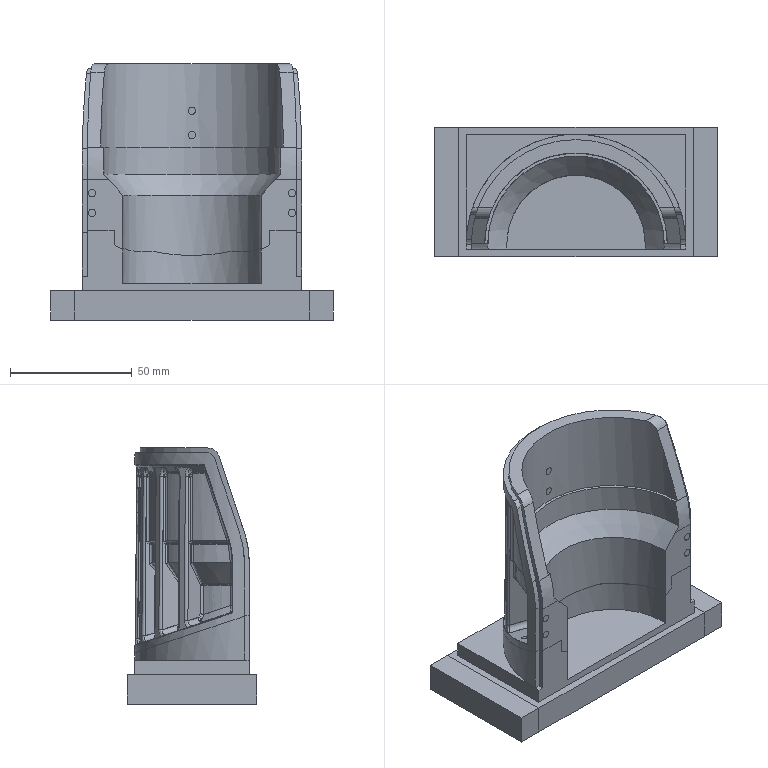NC program | NX | posted by the shop | part box 116 x 53 x 105 mm
Lines 43881 to 44922 of 572762:
T12 M6
;(T12:C-D4  D=4. R=0.)
;(XY=0.2mm Z=0.2mm)
G54 G90 D1
CYCLE832(0.04,_TOP_SURFACE_SMOOTH_ON+_ORI_SEMIFIN,1.)
CYCLE800(0,"AFMING",100000,57,0.,0.,0.,-90.,58.,0.,0.,0.,0.,-1,100.,1)
G0 X19.69 Y75.9713 S7000 M3 M8
Z103.43
X19.69 Y75.9713 Z103.43
Z35.088
G1 Z34.088 F3500.
G3 X19.4934 Y75.307 I1.003 J-.658
G1 X19.498 Y74.459
X19.485 Y73.938
G2 X19.302 Y73.304 I-2.561 J.393
X17.209 Y72.14 I-1.803 J.779
G1 X17.21 Y76.676
X19.486
X19.4934 Y75.307
X19.5154 Y74.973 Z34.094
X19.575 Y74.639 Z34.111
X19.6659 Y74.307 Z34.136
X19.784 Y73.978 Z34.166
X19.9245 Y73.653 Z34.2
X20.082 Y73.335 Z34.236
X20.434 Y72.712 Z34.3001
X20.827 Y72.073 Z34.345
X21.046 Y71.74 Z34.351
X21.2598 Y71.433 Z34.3445
X21.47 Y71.156 Z34.324
X21.676 Y70.912 Z34.292
X21.88 Y70.7056 Z34.246
X22.081 Y70.539 Z34.188
X22.208 Y70.455 Z34.145
X22.335 Y70.391 Z34.099
X22.462 Y70.349 Z34.05
X22.5896 Y70.331 Z34.002
X22.7184 Y70.339 Z33.955
X22.849 Y70.376 Z33.911
X22.981 Y70.442 Z33.871
X23.116 Y70.542 Z33.8374
X23.254 Y70.675 Z33.811
X23.395 Y70.846 Z33.795
X23.54 Y71.055 Z33.789
G3 X24.306 Y73.607 I-4.078 J2.6144
G1 Y76.676
G2 X24.675 Y77.542 I1.2 J0.0
G1 Z34.789
G0 X15.209 Y67.388
G1 Z33.789
X15.742 Y68.365
G2 X17.209 Y69.218 I1.16 J-.307
G3 X18.094 Y69.006 I5.026 J18.976
G2 X18.286 Y68.947 I-.253 J-1.173
G1 Z34.789
G0 X24.306 Y76.676 Z34.289
G1 Z33.789
X21.506
Y73.632
G2 X19.135 Y71.6517 I-2.044 J.038
X17.209 Y72.132 I3.1 J16.5422
G3 X15.705 Y71.345 I-.358 J-1.145
G1 Z34.789
G0 X15.791 Y33.438 Z34.49
G1 Z33.49
X16.008 Y33.976
G2 X17.209 Y35.175 I1.2 J-.001
G3 X18.554 Y35.201 I.037 J32.758
G1 X18.5556 Y35.216
G3 X18.627 Y38.0068 I-274.999 J8.4296
G2 X17.209 Y37.975 I-1.382 J29.926
G1 Y40.775
G3 X18.67 Y40.812 I.037 J27.1579
X18.685 Y43.353 I-275.114 J2.834
G1 X18.678 Y43.368
X18.693 Y43.374
G3 X18.903 Y43.631 I-1.417 J1.3685
G2 X17.209 Y43.575 I-1.6571 J24.3015
G1 Y46.375
G3 X19.277 Y46.471 I.037 J21.558
G1 X19.328 Y49.291
G2 X17.209 Y49.175 I-2.0824 J18.642
G1 Y51.975
G3 X19.379 Y52.118 I.037 J15.958
G1 X19.43 Y54.9575
G2 X17.209 Y54.775 I-2.184 J12.975
G1 Y57.575
G3 X19.4812 Y57.8191 I.037 J10.358
G1 X19.485 Y58.021
X19.536 Y60.069
G2 X19.534 Y60.7296 I54.9157 J.573
X17.209 Y60.375 I-2.288 J7.203
G1 Y63.175
G3 X19.589 Y63.792 I.037 J4.758
G2 X19.789 Y63.883 I.591 J-1.044
G1 Z34.49
G0 X27.205 Y77.875
G1 Z33.49
X26.777 Y77.876
G3 X25.577 Y76.676 I0.0 J-1.2
G1 Y72.434
G2 X23.121 Y70.4202 I-2.094 J.049
X19.564 Y71.126 I5.24 J35.731
G1 X19.464 Y70.86
X19.335 Y68.4635
X19.171 Y67.576
G2 X17.209 Y65.975 I-1.925 J.357
G3 X15.9867 Y64.798 I-.022 J-1.2
G1 Z34.49
G0 X28.507 Y77.819 Z34.191
G1 Z33.191
G3 X27.671 Y76.676 I.364 J-1.144
G1 Y71.791
G2 X25.513 Y69.7422 I-2.08 J.03
X23.1266 Y70.072 I.982 J15.906
G3 X22.458 Y70.025 I-.254 J-1.173
G1 Z34.191
G0 X30.015 Y77.781 Z33.892
G1 Z32.892
G3 X29.283 Y76.676 I.468 J-1.105
G1 Y71.284
G2 X27.108 Y69.227 I-2.1013 J.044
G1 X26.709 Y69.252
X26.07 Y69.3048
G2 X25.354 Y69.398 I.636 J7.696
G3 X24.708 Y69.3345 I-.21 J-1.181
G1 Z33.892
G0 X31.158 Y77.663 Z33.592
G1 Z32.592
G3 X30.64 Y76.676 I.682 J-.987
G1 Y70.845
G2 X28.714 Y68.806 I-2.042 J0.0
X26.859 Y68.917 I-.456 J7.948
G3 X26.213 Y68.855 I-.211 J-1.1813
G1 Z33.592
G0 X32.492 Y77.748 Z33.293
G1 Z32.293
G3 X31.831 Y76.676 I.54 J-1.072
G1 Y70.46
G2 X29.83 Y68.4 I-2.0607 J0.0
X28.315 Y68.456 I-.33 J11.492
G3 X27.742 Y68.375 I-.1237 J-1.194
G1 Z33.293
G0 Z36.49
X33.297 Y77.563
Z32.994
G1 Z31.994
G3 X32.905 Y76.676 I.808 J-.887
G1 Y70.107
G2 X31.073 Y68.056 I-2.064 J0.0
X30.297 Y68.033 I-.531 J4.693
X29.477 Y68.075 I-.178 J4.503
G3 X28.859 Y68.001 I-.171 J-1.188
G1 Z32.994
G0 Z36.191
X34.566 Y77.7567
Z32.695
G1 Z31.695
G3 X33.887 Y76.676 I.521 J-1.081
G1 Y69.766
G2 X32.307 Y67.794 I-2.021 J0.0
X30.503 Y67.73 I-1.072 J4.801
G3 X29.882 Y67.659 I-.178 J-1.187
G1 Z32.695
G0 Z36.191
X35.1794 Y77.554
Z32.396
G1 Z31.396
G3 X34.797 Y76.676 I.818 J-.878
G1 Y69.47
G2 X33.018 Y67.423 I-2.0666 J0.0
X32.29 Y67.368 I-.801 J5.699
G1 X32.035 Y67.363
G2 X31.522 Y67.39 I-.072 J3.478
G3 X30.92 Y67.313 I-.152 J-1.19
G1 Z32.396
G0 Z35.892
X36.232 Y77.705
Z32.097
G1 Z31.097
G3 X35.648 Y76.676 I.6165 J-1.03
G1 Y69.173
G2 X34.096 Y67.184 I-2.051 J0.0
X32.339 Y67.1 I-1.087 J4.335
G3 X31.724 Y67.032 I-.18 J-1.186
G1 Z32.097
G0 Z35.592
X36.874 Y77.592
Z31.798
G1 Z30.798
G3 X36.449 Y76.676 I.7746 J-.917
G1 Y68.902
G2 X34.283 Y66.803 I-2.134 J.034
X33.2339 Y66.7966 I-.545 J3.639
G3 X32.629 Y66.724 I-.164 J-1.189
G1 Z31.798
G0 Z35.293
X37.518 Y77.483
Z31.499
G1 Z30.499
G3 X37.2066 Y76.676 I.888 J-.807
G1 Y68.637
G2 X35.081 Y66.531 I-2.173 J.0671
X34.038 Y66.516 I-.57 J3.463
G3 X33.435 Y66.443 I-.162 J-1.189
G1 Z31.499
G0 Z34.994
X38.442 Y77.6613
Z31.2
G1 Z30.2
G3 X37.927 Y76.676 I.685 J-.985
G1 Y74.666
X37.944 Y74.2372 Z30.212
X37.9907 Y73.811 Z30.244
X38.06 Y73.389 Z30.291
X38.287 Y72.393 Z30.435
X38.525 Y71.408 Z30.562
X38.6 Y71.021 Z30.589
X38.652 Y70.649 Z30.597
X38.675 Y70.285 Z30.589
X38.666 Y69.924 Z30.562
X38.621 Y69.559 Z30.518
X38.5507 Y69.24 Z30.467
X38.451 Y68.913 Z30.408
X38.324 Y68.5805 Z30.348
X38.169 Y68.242 Z30.291
X37.988 Y67.899 Z30.244
X37.781 Y67.5517 Z30.212
X37.55 Y67.201 Z30.2
G2 X35.878 Y66.284 I-1.751 J1.209
X34.363 Y66.336 I-.644 J3.302
G1 X34.204 Y66.381
G3 X33.5108 Y66.369 I-.326 J-1.155
G1 Z31.2
G0 Z34.994
X39.108 Y77.646
Z30.901
G1 Z29.901
G3 X38.6141 Y76.676 I.706 J-.971
G1 Y68.1365
G2 X36.675 Y66.043 I-2.1266 J.025
X35.088 Y66.078 I-.72 J3.289
G1 X33.789 Y66.445
X33.5802 Y66.494 Z29.904
X33.4 Y66.5153 Z29.913
X33.246 Y66.512 Z29.926
X33.1174 Y66.485 Z29.944
X33.013 Y66.439 Z29.965
X32.931 Y66.374 Z29.987
X32.8702 Y66.294 Z30.011
X32.829 Y66.201 Z30.035
X32.806 Y66.097 Z30.058
X32.8 Y65.985 Z30.08
X32.81 Y65.866 Z30.0992
X32.8335 Y65.743 Z30.115
X32.903 Y65.53 Z30.132
X33.008 Y65.316 Z30.137
X33.146 Y65.104 Z30.129
X33.314 Y64.898 Z30.109
X33.512 Y64.701 Z30.077
X33.735 Y64.516 Z30.033
X33.984 Y64.348 Z29.978
X34.254 Y64.1981 Z29.912
X34.546 Y64.068 Z29.841
X34.86 Y63.958 Z29.77
X35.193 Y63.869 Z29.705
X35.545 Y63.801 Z29.651
X35.916 Y63.7547 Z29.615
X36.305 Y63.73 Z29.601
G3 X38.158 Y63.927 I.22 J6.75
X39.656 Y64.647 I-.9925 J3.985
G2 X39.884 Y64.784 I.728 J-.954
G1 Z30.601
G0 X39.907 Y77.735
G1 Z29.601
G3 X39.272 Y76.676 I.565 J-1.059
G1 Y67.899
G2 X37.674 Y65.868 I-2.107 J.013
X36.276 Y65.734 I-1.147 J4.613
X35.738 Y65.8415 I.4533 J3.667
G1 X33.554 Y66.459
G3 X32.862 Y66.447 I-.326 J-1.155
G1 Z30.601
G0 Z41.275
X19.701 Y5.95
Z35.088
G1 Z34.088
G3 X19.504 Y5.286 I1.003 J-.659
G1 X19.509 Y4.181
X19.5093 Y4.05
X17.209 Y4.051
Y8.835
G2 X19.18 Y7.795 I.228 J-1.957
X19.498 Y6.521 I-2.445 J-1.287
G1 X19.504 Y5.286
X19.522 Y5.0428 Z34.091
X19.57 Y4.814 Z34.101
X19.646 Y4.599 Z34.116
X19.748 Y4.397 Z34.136
X19.872 Y4.207 Z34.158
X20.016 Y4.03 Z34.183
X20.176 Y3.865 Z34.209
X20.35 Y3.7111 Z34.236
X20.535 Y3.568 Z34.2617
X20.728 Y3.436 Z34.286
X20.927 Y3.314 Z34.307
X21.128 Y3.202 Z34.3251
X21.473 Y3.032 Z34.345
X21.813 Y2.89 Z34.351
X22.145 Y2.777 Z34.3445
X22.466 Y2.694 Z34.324
X22.772 Y2.642 Z34.292
X23.06 Y2.622 Z34.246
X23.326 Y2.635 Z34.188
X23.482 Y2.662 Z34.145
X23.628 Y2.703 Z34.099
X23.761 Y2.762 Z34.05
X23.882 Y2.839 Z34.002
X23.99 Y2.937 Z33.955
X24.083 Y3.057 Z33.911
X24.161 Y3.201 Z33.871
X24.223 Y3.371 Z33.8374
X24.269 Y3.568 Z33.811
X24.296 Y3.794 Z33.795
X24.306 Y4.05 Z33.789
Y6.8
G3 X23.853 Y8.327 I-2.8 J0.0
G1 X23.761 Y8.469
X23.582 Y8.709 Z33.797
X23.3751 Y8.926 Z33.82
X23.142 Y9.1212 Z33.856
X22.885 Y9.295 Z33.902
X22.608 Y9.448 Z33.956
X22.311 Y9.581 Z34.016
X21.998 Y9.695 Z34.08
X21.6709 Y9.79 Z34.145
X21.332 Y9.8666 Z34.208
X20.984 Y9.926 Z34.269
X20.541 Y9.976 Z34.337
X20.092 Y10.002 Z34.395
X19.645 Y10.004 Z34.442
X19.206 Y9.985 Z34.476
X18.78 Y9.945 Z34.497
X18.373 Y9.887 Z34.504
X17.993 Y9.813 Z34.494
X17.644 Y9.7227 Z34.4681
X17.473 Y9.669 Z34.447
X17.314 Y9.612 Z34.421
X17.17 Y9.553 Z34.3902
X17.042 Y9.491 Z34.355
X16.932 Y9.428 Z34.317
X16.841 Y9.363 Z34.275
X16.772 Y9.299 Z34.229
X16.727 Y9.235 Z34.181
X16.706 Y9.1712 Z34.13
X16.712 Y9.109 Z34.077
X16.747 Y9.049 Z34.022
X16.8125 Y8.992 Z33.965
X16.91 Y8.938 Z33.907
X17.042 Y8.888 Z33.848
X17.209 Y8.842 Z33.789
G2 X19.932 Y8.763 I1.0281 J-11.584
G1 X20.331 Y8.607
X21.506 Y6.8
Y4.05
X21.499 Y3.881 Z33.792
X21.478 Y3.745 Z33.8
X21.444 Y3.643 Z33.813
X21.398 Y3.572 Z33.83
X21.339 Y3.53 Z33.851
X21.269 Y3.516 Z33.876
X21.188 Y3.529 Z33.9028
X21.096 Y3.566 Z33.932
X20.994 Y3.626 Z33.963
X20.883 Y3.707 Z33.996
X20.763 Y3.809 Z34.029
X20.635 Y3.928 Z34.0624
X20.354 Y4.217 Z34.127
X19.83 Y4.808 Z34.219
X19.529 Y5.164 Z34.258
X19.24 Y5.512 Z34.287
X18.8864 Y5.949 Z34.3114
X18.185 Y6.844 Z34.325
X17.6346 Y7.583 Z34.289
X17.38 Y7.941 Z34.25
X17.24 Y8.144 Z34.22
X17.111 Y8.3359 Z34.186
X16.996 Y8.517 Z34.147
X16.895 Y8.685 Z34.104
X16.81 Y8.839 Z34.058
X16.743 Y8.979 Z34.009
X16.696 Y9.1028 Z33.9573
X16.67 Y9.21 Z33.903
X16.666 Y9.298 Z33.847
X16.686 Y9.368 Z33.789
X16.733 Y9.417 Z33.73
X16.8065 Y9.445 Z33.67
X16.909 Y9.45 Z33.6101
X17.043 Y9.432 Z33.55
X17.209 Y9.389 Z33.49
G2 X21.454 Y9.282 I1.001 J-44.449
X24.235 Y8.7 I-.781 J-10.677
X25.577 Y6.803 I-.6694 J-1.897
G1 Y4.05
G3 X26.777 Y2.85 I1.2 J0.0
G1 X27.196
Z34.49
G0 X19.36 Y21.836 Z34.191
G1 Z33.191
G3 X19.16 Y21.823 I-.024 J-1.2
G2 X17.209 Y21.68 I-1.935 J13.052
G1 Y24.4803
G3 X19.464 Y24.724 I.016 J10.395
X19.589 Y25.379 I-1.819 J.687
X19.626 Y27.67 I-4989.184 J82.04
G2 X17.209 Y27.2803 I-2.402 J7.205
G1 Y30.08
G3 X19.674 Y30.754 I.015 J4.795
G2 X19.876 Y30.85 I.613 J-1.031
G1 Z34.191
G0 X21.112 Y70.402
G1 Z33.191
G3 X20.528 Y70.775 I-.91 J-.782
G1 X20.064 Y70.9062
X20.057 Y70.86
X19.932 Y60.194
G2 X19.533 Y39.529 I-1190.043 J12.6214
G1 X19.3343 Y35.317
X19.256 Y34.917
X19.135 Y34.309
G2 X17.209 Y32.88 I-1.913 J.567
G3 X16.001 Y31.688 I-.008 J-1.2
G1 Z34.191
G0 X17.209 Y21.68 Z33.691
G1 Z33.191
Y20.888
G2 X19.159 Y20.89 I1.024 J-58.148
G1 X19.156 Y18.089
G3 X17.209 Y18.088 I-.923 J-55.3497
G1 Y15.287
G2 X19.153 Y15.289 I1.024 J-52.547
G1 X19.151 Y12.489
G3 X17.209 Y12.487 I-.918 J-49.749
G1 Y9.686
G2 X23.919 Y9.3518 I1.025 J-46.946
G1 X24.317 Y9.301
G2 X26.534 Y8.626 I-.967 J-7.149
X27.671 Y6.801 I-.898 J-1.825
G1 Y4.05
G3 X28.871 Y2.85 I1.2 J0.0
G1 X29.138
Z34.191
G0 X21.299 Y70.296 Z33.892
G1 Z32.892
G3 X20.715 Y70.669 I-.91 J-.782
G1 X20.284 Y70.791
G2 X20.033 Y35.716 I-6875.221 J31.72
X19.829 Y19.935 I-2438.65 J23.532
G3 X20.018 Y19.268 I1.2 J-.019
G1 Z33.892
G0 X21.631 Y70.15 Z33.592
G1 Z32.592
G3 X21.047 Y70.523 I-.91 J-.782
G1 X20.395 Y70.707
G2 X20.1787 Y19.519 I-9999.986 J16.69
G3 X20.374 Y18.854 I1.2 J-.008
G1 Z33.592
G0 X29.853 Y12.247 Z33.892
G1 Z32.892
G2 X29.569 Y12.385 I.378 J1.139
G3 X28.609 Y12.841 I-2.1 J-3.183
X26.572 Y12.97 I-1.282 J-4.092
G1 X26.199 Y12.92 Z32.901
X25.82 Y12.899 Z32.926
X25.439 Y12.901 Z32.964
X25.059 Y12.924 Z33.011
X24.1243 Y13.034 Z33.1406
X23.167 Y13.17 Z33.254
X22.752 Y13.217 Z33.28
X22.355 Y13.244 Z33.289
X21.971 Y13.2452 Z33.28
X21.594 Y13.215 Z33.254
X21.22 Y13.148 Z33.21
X21.032 Y13.098 Z33.181
X20.846 Y13.037 Z33.149
X20.665 Y12.963 Z33.115
X20.491 Y12.875 Z33.08
X20.3269 Y12.771 Z33.0449
X20.175 Y12.652 Z33.011
X20.039 Y12.516 Z32.979
X19.921 Y12.3608 Z32.95
X19.823 Y12.187 Z32.926
X19.7481 Y11.992 Z32.908
X19.699 Y11.777 Z32.896
X19.679 Y11.538 Z32.892
X19.676 Y11.355
G3 X20.126 Y9.958 I2.449 J.018
G2 X25.16 Y9.482 I-1.975 J-47.78
X28.011 Y10.932 I2.167 J-.733
X29.283 Y9.202 I-.542 J-1.731
G1 Y4.05
G3 X30.01 Y2.9474 I1.2 J0.0
G1 Z33.892
G0 X31.338 Y16.025 Z33.592
G1 Z32.592
G2 X31.079 Y16.178 I.475 J1.102
G3 X27.96 Y16.968 I-2.4656 J-3.183
X27.39 Y16.149 I1.2807 J-1.4969
G1 X26.874 Y14.526
X26.868 Y14.515
G3 X26.519 Y13.956 I1.353 J-1.232
G1 X25.66 Y11.783
G2 X26.893 Y14.067 I19.062 J-8.8253
X30.64 Y12.995 I1.72 J-1.072
G1 Y4.05
G3 X31.285 Y2.986 I1.2 J0.0
G1 Z33.592
G0 X26.5795 Y15.217 Z33.293
G1 Z32.293
G3 X27.028 Y15.713 I-.631 J1.021
G2 X28.15 Y17.638 I13.333 J-6.481
X31.831 Y16.494 I1.663 J-1.145
G1 Y4.05
G3 X32.468 Y2.991 I1.2 J0.0
G1 Z33.293
G0 X27.69 Y18.528 Z32.994
G1 Z31.994
G3 X28.135 Y19.022 I-.633 J1.019
G2 X29.21 Y20.846 I11.885 J-5.777
X32.905 Y19.677 I1.662 J-1.169
G1 Y4.423
G2 X32.877 Y4.05 I-4.578 J.154
G3 X33.034 Y3.305 I1.192 J-.138
G1 Z32.994
G0 X28.687 Y21.55 Z32.695
G1 Z31.695
G3 X29.127 Y22.044 I-.641 J1.014
G2 X30.215 Y23.851 I10.1645 J-4.891
X33.887 Y22.6429 I1.637 J-1.208
G1 Y7.385
G2 X33.635 Y5.943 I-6.9813 J.479
X33.047 Y4.05 I-41.377 J11.812
G3 X33.054 Y3.265 I1.138 J-.3822
G1 Z32.695
G0 Z36.191
X29.645 Y24.4648
Z32.396
G1 Z31.396
G3 X30.084 Y24.954 I-.64 J1.015
G2 X31.149 Y26.668 I8.872 J-4.325
X34.797 Y25.422 I1.6114 J-1.246
G1 Y10.164
G2 X34.515 Y8.596 I-7.166 J.4798
X33.945 Y6.782 I-59.468 J17.69
G1 X33.329 Y4.922
G2 X33.236 Y4.628 I-41.071 J12.833
G3 X33.222 Y3.944 I1.143 J-.366
G1 Z32.396
G0 Z35.892
X30.582 Y27.323
Z32.097
G1 Z31.097
G3 X31.022 Y27.801 I-.629 J1.0217
G2 X32.0889 Y29.39 I7.086 J-3.602
X35.648 Y28.067 I1.5338 J-1.323
G1 Y12.792
G2 X35.53 Y11.925 I-8.809 J.755
G3 X35.615 Y11.215 I1.18 J-.22
G1 Z32.097
G0 Z35.592
X31.382 Y29.838
Z31.798
G1 Z30.798
G3 X31.8177 Y30.317 I-.638 J1.017
G2 X32.89 Y31.908 I6.693 J-3.352
X36.449 Y30.566 I1.526 J-1.343
G1 Y15.293
G2 X36.228 Y13.937 I-6.5184 J.365
X35.889 Y12.791 I-27.169 J7.426
X35.699 Y12.199 I-782.528 J250.0204
G3 X35.7039 Y11.4526 I1.1428 J-.366
G1 Z31.798
G0 Z35.293
X32.251 Y32.516
Z31.499
G1 Z30.499
G3 X32.697 Y32.978 I-.61 J1.0334
G2 X33.689 Y34.354 I5.8 J-3.138
X37.2066 Y32.961 I1.483 J-1.392
G1 Y17.686
G2 X36.824 Y15.748 I-8.379 J.648
X35.957 Y13.008 I-723.091 J227.259
G3 X35.949 Y12.323 I1.146 J-.356
G1 Z31.499
G0 Z35.293
X32.919 Y34.699
Z31.2
G1 Z30.2
G3 X33.352 Y35.172 I-.636 J1.018
G2 X34.377 Y36.643 I5.8269 J-2.967
X37.927 Y35.254 I1.503 J-1.389
G1 Y34.157
X37.982 Y33.964 Z30.269
X38.012 Y33.801 Z30.339
X38.016 Y33.668 Z30.408
X37.997 Y33.562 Z30.476
X37.955 Y33.482 Z30.544
X37.892 Y33.426 Z30.6087
X37.809 Y33.392 Z30.671
X37.707 Y33.38 Z30.7306
X37.5876 Y33.386 Z30.786
X37.452 Y33.41 Z30.838
X37.301 Y33.449 Z30.884
X37.137 Y33.503 Z30.9249
X36.96 Y33.569 Z30.96
X36.649 Y33.699 Z31.002
X36.316 Y33.855 Z31.028
X35.97 Y34.033 Z31.036
X35.62 Y34.231 Z31.027
X35.273 Y34.446 Z31.001
X34.939 Y34.675 Z30.958
X34.6245 Y34.914 Z30.899
X34.339 Y35.161 Z30.823
X34.1693 Y35.329 Z30.763
X34.018 Y35.499 Z30.697
X33.887 Y35.67 Z30.626
X33.779 Y35.843 Z30.55
X33.695 Y36.017 Z30.471
X33.638 Y36.192 Z30.39
X33.6087 Y36.367 Z30.306
X33.6103 Y36.543 Z30.223
X33.644 Y36.719 Z30.139
X33.713 Y36.895 Z30.057
X33.818 Y37.0701 Z29.977
X33.961 Y37.245 Z29.901
G2 X35.011 Y38.881 I6.467 J-2.995
X38.6141 Y37.55 I1.556 J-1.33
G1 Y22.198
G2 X38.317 Y20.531 I-7.512 J.478
G3 X38.324 Y19.823 I1.15 J-.342
G1 Z30.901
G0 X36.713 Y48.173 Z30.601
G1 Z29.601
G3 X37.091 Y48.12 I.351 J1.147
G2 X38.676 Y47.989 I.17 J-7.609
X39.6966 Y46.442 I-.941 J-1.731
G1 X39.697 Y44.659
G3 X35.692 Y45.059 I-2.437 J-4.148
G2 X35.6 Y44.04 I-43.713 J3.416
G1 X35.265 Y41.708
G2 X34.979 Y40.941 I-1.891 J.268
X34.718 Y40.011 I-50.034 J13.512
X35.618 Y41.671 I7.423 J-2.947
X39.272 Y40.511 I1.643 J-1.16
G1 Y24.337
G2 X38.936 Y22.537 I-7.8743 J.539
X38.444 Y20.935 I-776.206 J237.345
G3 X38.44 Y20.243 I1.147 J-.353
G1 Z30.601
G0 Z34.097
X35.414 Y57.192
Z30.302
G1 Z29.302
G2 X35.614 Y57.18 I.027 J-1.1997
G3 X39.211 Y57.248 I1.591 J10.9108
X40.18 Y57.43 I-1.461 J10.451
G1 X40.1806 Y60.338
G2 X38.762 Y60.013 I-2.43 J7.362
X35.614 Y60.02 I-1.558 J8.077
G1 Y62.904
X35.632 Y62.897
G3 X38.315 Y62.779 I1.5727 J5.193
X40.181 Y63.384 I-.565 J4.921
G2 X40.381 Y63.474 I.589 J-1.046
G1 Z30.302
G0 X40.384 Y77.637
G1 Z29.302
G3 X39.903 Y76.676 I.719 J-.961
G1 Y67.669
G2 X37.871 Y65.55 I-2.153 J.031
X36.476 Y65.568 I-.665 J2.541
G1 X36.2764 Y65.636
X33.371 Y66.458
G3 X32.679 Y66.446 I-.326 J-1.155
G1 Z30.302
G0 X40.38 Y56.6
G1 Z29.302
G2 X40.18 Y56.6286 I.067 J1.198
G3 X38.207 Y56.883 I-2.3135 J-10.15
X35.614 Y56.642 I-.342 J-10.404
G1 Y53.748
G2 X40.179 Y53.729 I2.253 J-7.269
G1 X40.179 Y50.697
G3 X35.614 Y50.729 I-2.312 J-4.218
G1 X35.384 Y50.588 Z29.307
X35.1766 Y50.422 Z29.321
X34.991 Y50.233 Z29.3432
X34.825 Y50.022 Z29.371
X34.68 Y49.791 Z29.404
X34.554 Y49.543 Z29.44
X34.446 Y49.279 Z29.478
X34.355 Y49.001 Z29.517
X34.282 Y48.71 Z29.554
X34.224 Y48.409 Z29.5892
X34.182 Y48.099 Z29.621
X34.147 Y47.663 Z29.655
X34.137 Y47.219 Z29.68
X34.151 Y46.776 Z29.695
X34.187 Y46.337 Z29.7
X34.243 Y45.91 Z29.695
X34.316 Y45.501 Z29.68
X34.406 Y45.116 Z29.655
X34.511 Y44.76 Z29.621
X34.572 Y44.585 Z29.598
X34.636 Y44.422 Z29.573
X34.702 Y44.274 Z29.547
X34.77 Y44.141 Z29.519
X34.8385 Y44.027 Z29.491
X34.908 Y43.933 Z29.463
X34.977 Y43.861 Z29.435
X35.0445 Y43.813 Z29.409
X35.111 Y43.7908 Z29.384
X35.175 Y43.797 Z29.361
X35.236 Y43.833 Z29.342
X35.294 Y43.902 Z29.325
X35.348 Y44.004 Z29.313
X35.397 Y44.142 Z29.305
X35.44 Y44.318 Z29.302
G2 X35.811 Y46.099 I593.181 J-122.651
G1 X35.8654 Y46.669
G2 X39.8754 Y46.538 I2.001 J-.19
G1 X39.905 Y45.5277
X39.903 Y45.478
Y26.41
G2 X39.657 Y24.933 I-6.317 J.296
G1 X39.546 Y24.534
X38.907 Y22.442
X38.861 Y22.28 Z29.305
X38.831 Y22.149 Z29.313
X38.815 Y22.05 Z29.326
X38.814 Y21.98 Z29.344
X38.825 Y21.938 Z29.365
X38.849 Y21.923 Z29.389
X38.883 Y21.932 Z29.416
X38.927 Y21.966 Z29.446
X38.98 Y22.0211 Z29.477
X39.041 Y22.0971 Z29.509
X39.109 Y22.192 Z29.543
X39.183 Y22.305 Z29.576
X39.306 Y22.512 Z29.626
X39.3896 Y22.662 Z29.658
X39.517 Y22.904 Z29.701
X39.673 Y23.2294 Z29.747
X39.83 Y23.581 Z29.785
X39.983 Y23.952 Z29.814
X40.132 Y24.3364 Z29.834
X40.272 Y24.727 Z29.843
X40.401 Y25.119 Z29.842
X40.516 Y25.504 Z29.828
X40.615 Y25.876 Z29.802
X40.695 Y26.229 Z29.764
X40.733 Y26.4285 Z29.734
X40.763 Y26.617 Z29.699
X40.785 Y26.7919 Z29.66
X40.7979 Y26.9516 Z29.618
X40.802 Y27.094 Z29.572
X40.798 Y27.2169 Z29.523
X40.784 Y27.318 Z29.4708
X40.761 Y27.3966 Z29.417
X40.728 Y27.449 Z29.36
X40.685 Y27.475 Z29.303
X40.632 Y27.47 Z29.244
X40.569 Y27.435 Z29.184
X40.495 Y27.365 Z29.1236
X40.411 Y27.261 Z29.063
X40.315 Y27.118 Z29.003
G2 X40.208 Y26.731 I-6.928 J1.705
X39.556 Y24.572 I-815.3648 J244.917
G1 X39.546 Y24.534
X39.512 Y24.423
X39.459 Y24.236 Z29.007
X39.425 Y24.083 Z29.017
X39.409 Y23.9636 Z29.034
X39.408 Y23.875 Z29.056
X39.4223 Y23.8155 Z29.083
X39.45 Y23.784 Z29.113
X39.489 Y23.778 Z29.147
X39.538 Y23.796 Z29.182
X39.597 Y23.837 Z29.22
X39.663 Y23.899 Z29.258
X39.7359 Y23.98 Z29.296
X39.813 Y24.078 Z29.333
X39.894 Y24.192 Z29.369
X39.977 Y24.3191 Z29.402
X40.124 Y24.571 Z29.454
X40.269 Y24.852 Z29.4944
X40.41 Y25.154 Z29.524
X40.541 Y25.469 Z29.541
X40.66 Y25.789 Z29.545
X40.762 Y26.106 Z29.534
X40.845 Y26.411 Z29.507
X40.905 Y26.698 Z29.464
X40.927 Y26.849 Z29.432
X40.939 Y26.99 Z29.395
X40.943 Y27.118 Z29.353
X40.937 Y27.23 Z29.306
X40.922 Y27.326 Z29.2555
X40.896 Y27.402 Z29.202
X40.861 Y27.457 Z29.145
X40.815 Y27.49 Z29.086
X40.7592 Y27.497 Z29.024
X40.692 Y27.476 Z28.962
X40.615 Y27.427 Z28.898
X40.526 Y27.346 Z28.833
X40.426 Y27.232 Z28.768
X40.315 Y27.083 Z28.704
G2 X40.134 Y26.48 I-824.533 J247.438
G3 X40.134 Y25.788 I1.149 J-.346
G1 Z29.704
G0 Z33.499
X35.144 Y63.531
Z30.003
G1 Z29.003
G3 X35.344 Y64.194 I-1. J.663
G1 Y65.847
X33.196 Y66.454
X33.038 Y66.489 Z29.005
X32.905 Y66.499 Z29.011
X32.794 Y66.486 Z29.021
X32.706 Y66.452 Z29.033
X32.639 Y66.398 Z29.0469
X32.591 Y66.327 Z29.063
X32.562 Y66.24 Z29.0793
X32.549 Y66.14 Z29.096
X32.5529 Y66.028 Z29.113
X32.571 Y65.906 Z29.129
X32.603 Y65.7771 Z29.144
X32.647 Y65.642 Z29.157
X32.702 Y65.503 Z29.167
X32.829 Y65.239 Z29.178
X32.986 Y64.974 Z29.178
X33.167 Y64.714 Z29.168
X33.367 Y64.465 Z29.148
X33.584 Y64.232 Z29.119
X33.811 Y64.02 Z29.079
X34.044 Y63.837 Z29.03
X34.171 Y63.752 Z29.
X34.297 Y63.679 Z28.968
X34.42 Y63.618 Z28.935
X34.538 Y63.573 Z28.901
X34.651 Y63.5436 Z28.8677
X34.757 Y63.533 Z28.836
X34.8536 Y63.5412 Z28.805
X34.9397 Y63.571 Z28.777
X35.014 Y63.624 Z28.753
X35.074 Y63.702 Z28.733
X35.119 Y63.807 Z28.717
X35.147 Y63.939 Z28.708
X35.157 Y64.101 Z28.704
Y65.847
X33.077 Y66.435
X32.91 Y66.471 Z28.707
X32.77 Y66.479 Z28.713
X32.658 Y66.459 Z28.7239
X32.57 Y66.416 Z28.737
X32.505 Y66.351 Z28.753
X32.463 Y66.267 Z28.77
X32.441 Y66.166 Z28.788
X32.438 Y66.051 Z28.806
X32.452 Y65.923 Z28.823
X32.481 Y65.786 Z28.839
X32.526 Y65.642 Z28.853
X32.5823 Y65.493 Z28.864
X32.705 Y65.233 Z28.874
X32.857 Y64.971 Z28.874
X33.032 Y64.714 Z28.864
X33.228 Y64.467 Z28.844
X33.438 Y64.236 Z28.814
X33.659 Y64.027 Z28.775
X33.886 Y63.845 Z28.726
X34.009 Y63.761 Z28.697
X34.132 Y63.688 Z28.665
X34.252 Y63.628 Z28.632
X34.367 Y63.582 Z28.599
X34.4773 Y63.553 Z28.566
X34.58 Y63.541 Z28.535
X34.674 Y63.549 Z28.505
X34.758 Y63.578 Z28.4773
X34.8304 Y63.63 Z28.453
X34.889 Y63.706 Z28.433
X34.933 Y63.809 Z28.418
X34.961 Y63.938 Z28.408
X34.97 Y64.098 Z28.405
Y65.847
X32.89 Y66.435
X32.733 Y66.47 Z28.407
X32.601 Y66.48 Z28.413
X32.491 Y66.466 Z28.422
X32.403 Y66.432 Z28.4341
X32.336 Y66.378 Z28.448
X32.2876 Y66.307 Z28.464
X32.257 Y66.22 Z28.48
X32.244 Y66.12 Z28.497
X32.247 Y66.008 Z28.513
X32.263 Y65.887 Z28.529
X32.293 Y65.758 Z28.544
X32.335 Y65.623 Z28.556
X32.388 Y65.484 Z28.566
X32.511 Y65.2212 Z28.577
X32.663 Y64.957 Z28.577
X32.8389 Y64.697 Z28.567
X33.035 Y64.448 Z28.547
X33.245 Y64.215 Z28.517
X33.467 Y64.004 Z28.478
X33.695 Y63.8201 Z28.429
X33.819 Y63.735 Z28.399
X33.9417 Y63.661 Z28.367
X34.062 Y63.6 Z28.334
X34.178 Y63.554 Z28.301
X34.288 Y63.5241 Z28.268
X34.392 Y63.512 Z28.236
X34.4863 Y63.52 Z28.2061
X34.571 Y63.549 Z28.1786
X34.643 Y63.601 Z28.154
X34.702 Y63.6775 Z28.134
X34.746 Y63.78 Z28.119
X34.7736 Y63.911 Z28.109
X34.783 Y64.071 Z28.106
Y65.847
X32.5986 Y66.465
X32.439 Y66.5 Z28.108
X32.304 Y66.51 Z28.114
X32.193 Y66.497 Z28.124
X32.104 Y66.463 Z28.136
X32.036 Y66.409 Z28.15
X31.989 Y66.337 Z28.166
X31.959 Y66.25 Z28.183
X31.947 Y66.149 Z28.2
X31.952 Y66.0366 Z28.217
X31.971 Y65.914 Z28.234
X32.003 Y65.784 Z28.249
X32.048 Y65.648 Z28.262
X32.104 Y65.508 Z28.272
X32.234 Y65.243 Z28.2833
X32.393 Y64.977 Z28.284
X32.577 Y64.715 Z28.274
X32.781 Y64.4641 Z28.254
X33.001 Y64.23 Z28.224
X33.2312 Y64.017 Z28.184
X33.468 Y63.833 Z28.135
X33.597 Y63.748 Z28.105
X33.724 Y63.674 Z28.072
X33.849 Y63.614 Z28.039
X33.969 Y63.568 Z28.005
X34.084 Y63.539 Z27.972
X34.191 Y63.528 Z27.939
X34.289 Y63.537 Z27.909
X34.376 Y63.568 Z27.8807
X34.451 Y63.622 Z27.856
X34.512 Y63.701 Z27.8357
X34.5578 Y63.806 Z27.82
X34.586 Y63.9402 Z27.81
X34.596 Y64.104 Z27.807
Y65.847
X32.512 Y66.436
X32.346 Y66.472 Z27.809
X32.207 Y66.48 Z27.816
X32.095 Y66.461 Z27.826
X32.008 Y66.418 Z27.84
X31.944 Y66.353 Z27.8554
X31.902 Y66.27 Z27.872
X31.881 Y66.17 Z27.89
X31.878 Y66.0551 Z27.908
X31.892 Y65.929 Z27.925
X31.922 Y65.793 Z27.941
X31.966 Y65.65 Z27.954
X32.023 Y65.502 Z27.965
X32.147 Y65.243 Z27.975
X32.298 Y64.983 Z27.975
X32.474 Y64.728 Z27.965
X32.669 Y64.4829 Z27.945
X32.879 Y64.254 Z27.916
X33.1 Y64.046 Z27.876
X33.327 Y63.866 Z27.828
X33.45 Y63.7826 Z27.798
X33.572 Y63.71 Z27.767
X33.692 Y63.651 Z27.734
X33.807 Y63.606 Z27.701
X33.917 Y63.577 Z27.668
X34.02 Y63.566 Z27.6368
X34.114 Y63.574 Z27.607
X34.198 Y63.603 Z27.58
X34.27 Y63.654 Z27.556
X34.329 Y63.73 Z27.536
X34.372 Y63.832 Z27.521
X34.4 Y63.962 Z27.511
X34.409 Y64.12 Z27.508
Y65.847
X32.307 Y66.441
X32.151 Y66.476 Z27.51
X32.019 Y66.4858 Z27.516
X31.91 Y66.473 Z27.525
X31.823 Y66.4385 Z27.537
X31.756 Y66.385 Z27.551
X31.709 Y66.315 Z27.566
X31.6796 Y66.229 Z27.582
X31.667 Y66.13 Z27.599
X31.67 Y66.019 Z27.6156
X31.688 Y65.899 Z27.631
X31.718 Y65.771 Z27.646
X31.761 Y65.637 Z27.658
X31.815 Y65.499 Z27.668
X31.939 Y65.238 Z27.679
X32.092 Y64.976 Z27.679
X32.269 Y64.719 Z27.6687
X32.466 Y64.472 Z27.649
X32.678 Y64.241 Z27.619
X32.901 Y64.032 Z27.58
X33.13 Y63.85 Z27.531
X33.255 Y63.766 Z27.5012
X33.378 Y63.693 Z27.469
X33.499 Y63.633 Z27.437
X33.615 Y63.588 Z27.403
X33.726 Y63.5585 Z27.37
X33.83 Y63.547 Z27.339
X33.9246 Y63.555 Z27.309
X34.009 Y63.585 Z27.281
X34.082 Y63.637 Z27.257
X34.141 Y63.714 Z27.237
X34.185 Y63.816 Z27.222
X34.213 Y63.947 Z27.212
X34.222 Y64.107 Z27.209
Y65.847
X32.116 Y66.443
X31.961 Y66.477 Z27.211
X31.8289 Y66.487 Z27.217
X31.72 Y66.474 Z27.226
X31.633 Y66.44 Z27.238
X31.567 Y66.387 Z27.251
X31.519 Y66.316 Z27.2668
X31.49 Y66.231 Z27.283
X31.478 Y66.132 Z27.3